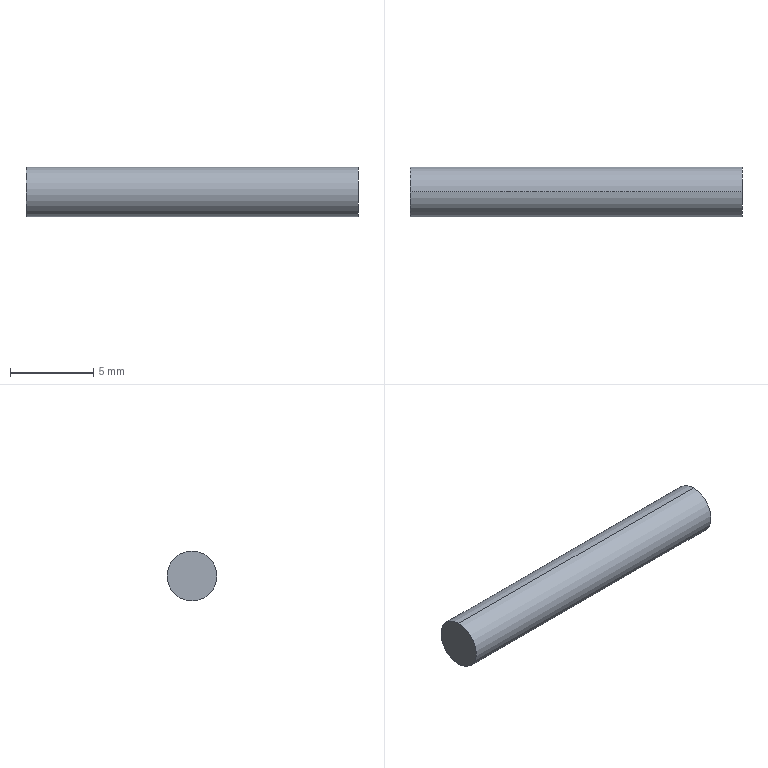Part | SolidWorks | features Extrusion 1 | 1 solid | 4 faces | box 20 x 3 x 3 mm | volume 141.372 mm3 | cylinder 2 | plane 2 | commonest cylinder face diameters 3 x2
STEP:
#1=CARTESIAN_POINT('',(20.,0.,-1.5));
#2=VERTEX_POINT('',#1);
#3=CARTESIAN_POINT('',(20.,0.,1.5));
#4=VERTEX_POINT('',#3);
#5=CARTESIAN_POINT('',(20.,0.,0.));
#6=DIRECTION('',(1.,0.,0.));
#7=DIRECTION('',(0.,0.,-1.));
#8=AXIS2_PLACEMENT_3D('',#5,#6,#7);
#9=CIRCLE('',#8,1.5);
#10=EDGE_CURVE('',#2,#4,#9,.T.);
#11=ORIENTED_EDGE('',*,*,#10,.F.);
#12=CARTESIAN_POINT('',(0.,0.,-1.5));
#13=VERTEX_POINT('',#12);
#14=CARTESIAN_POINT('',(20.,0.,-1.5));
#15=DIRECTION('',(-1.,0.,0.));
#16=VECTOR('',#15,1000.);
#17=LINE('',#14,#16);
#18=EDGE_CURVE('',#2,#13,#17,.T.);
#19=ORIENTED_EDGE('',*,*,#18,.T.);
#20=CARTESIAN_POINT('',(0.,0.,1.5));
#21=VERTEX_POINT('',#20);
#22=CARTESIAN_POINT('',(0.,0.,0.));
#23=DIRECTION('',(1.,0.,0.));
#24=DIRECTION('',(0.,0.,-1.));
#25=AXIS2_PLACEMENT_3D('',#22,#23,#24);
#26=CIRCLE('',#25,1.5);
#27=EDGE_CURVE('',#13,#21,#26,.T.);
#28=ORIENTED_EDGE('',*,*,#27,.T.);
#29=CARTESIAN_POINT('',(20.,0.,1.5));
#30=DIRECTION('',(-1.,0.,0.));
#31=VECTOR('',#30,1000.);
#32=LINE('',#29,#31);
#33=EDGE_CURVE('',#4,#21,#32,.T.);
#34=ORIENTED_EDGE('',*,*,#33,.F.);
#35=EDGE_LOOP('',(#11,#19,#28,#34));
#36=FACE_OUTER_BOUND('',#35,.T.);
#37=CARTESIAN_POINT('',(20.,0.,0.));
#38=DIRECTION('',(-1.,0.,0.));
#39=DIRECTION('',(0.,0.,1.));
#40=AXIS2_PLACEMENT_3D('',#37,#38,#39);
#41=CYLINDRICAL_SURFACE('',#40,1.5);
#42=ADVANCED_FACE('',(#36),#41,.T.);
#43=ORIENTED_EDGE('',*,*,#18,.F.);
#44=CARTESIAN_POINT('',(20.,0.,0.));
#45=DIRECTION('',(1.,0.,0.));
#46=DIRECTION('',(0.,0.,-1.));
#47=AXIS2_PLACEMENT_3D('',#44,#45,#46);
#48=CIRCLE('',#47,1.5);
#49=EDGE_CURVE('',#4,#2,#48,.T.);
#50=ORIENTED_EDGE('',*,*,#49,.F.);
#51=ORIENTED_EDGE('',*,*,#33,.T.);
#52=CARTESIAN_POINT('',(0.,0.,0.));
#53=DIRECTION('',(1.,0.,0.));
#54=DIRECTION('',(0.,0.,-1.));
#55=AXIS2_PLACEMENT_3D('',#52,#53,#54);
#56=CIRCLE('',#55,1.5);
#57=EDGE_CURVE('',#21,#13,#56,.T.);
#58=ORIENTED_EDGE('',*,*,#57,.T.);
#59=EDGE_LOOP('',(#43,#50,#51,#58));
#60=FACE_OUTER_BOUND('',#59,.T.);
#61=CARTESIAN_POINT('',(20.,0.,0.));
#62=DIRECTION('',(-1.,0.,0.));
#63=DIRECTION('',(0.,0.,1.));
#64=AXIS2_PLACEMENT_3D('',#61,#62,#63);
#65=CYLINDRICAL_SURFACE('',#64,1.5);
#66=ADVANCED_FACE('',(#60),#65,.T.);
#67=ORIENTED_EDGE('',*,*,#49,.T.);
#68=ORIENTED_EDGE('',*,*,#10,.T.);
#69=EDGE_LOOP('',(#67,#68));
#70=FACE_OUTER_BOUND('',#69,.T.);
#71=CARTESIAN_POINT('',(20.,0.,0.));
#72=DIRECTION('',(1.,0.,0.));
#73=DIRECTION('',(0.,0.,-1.));
#74=AXIS2_PLACEMENT_3D('',#71,#72,#73);
#75=PLANE('',#74);
#76=ADVANCED_FACE('',(#70),#75,.T.);
#77=ORIENTED_EDGE('',*,*,#57,.F.);
#78=ORIENTED_EDGE('',*,*,#27,.F.);
#79=EDGE_LOOP('',(#77,#78));
#80=FACE_OUTER_BOUND('',#79,.T.);
#81=CARTESIAN_POINT('',(0.,0.,0.));
#82=DIRECTION('',(1.,0.,0.));
#83=DIRECTION('',(0.,0.,-1.));
#84=AXIS2_PLACEMENT_3D('',#81,#82,#83);
#85=PLANE('',#84);
#86=ADVANCED_FACE('',(#80),#85,.F.);
#87=CLOSED_SHELL('',(#42,#66,#76,#86));
#88=MANIFOLD_SOLID_BREP('',#87);
#89=CARTESIAN_POINT('',(0.,0.,0.));
#90=DIRECTION('',(0.,0.,1.));
#91=DIRECTION('',(1.,0.,0.));
#92=AXIS2_PLACEMENT_3D('',#89,#90,#91);
#93=(LENGTH_UNIT()NAMED_UNIT(*)SI_UNIT(.MILLI.,.METRE.));
#94=UNCERTAINTY_MEASURE_WITH_UNIT(LENGTH_MEASURE(0.00001),#93,'','');
#95=(NAMED_UNIT(*)PLANE_ANGLE_UNIT()SI_UNIT($,.RADIAN.));
#96=(NAMED_UNIT(*)SI_UNIT($,.STERADIAN.)SOLID_ANGLE_UNIT());
#97=(GEOMETRIC_REPRESENTATION_CONTEXT(3)GLOBAL_UNCERTAINTY_ASSIGNED_CONTEXT((#94))GLOBAL_UNIT_ASSIGNED_CONTEXT((#93,#95,#96))REPRESENTATION_CONTEXT('',''));
#98=ADVANCED_BREP_SHAPE_REPRESENTATION('',(#88,#92),#97);